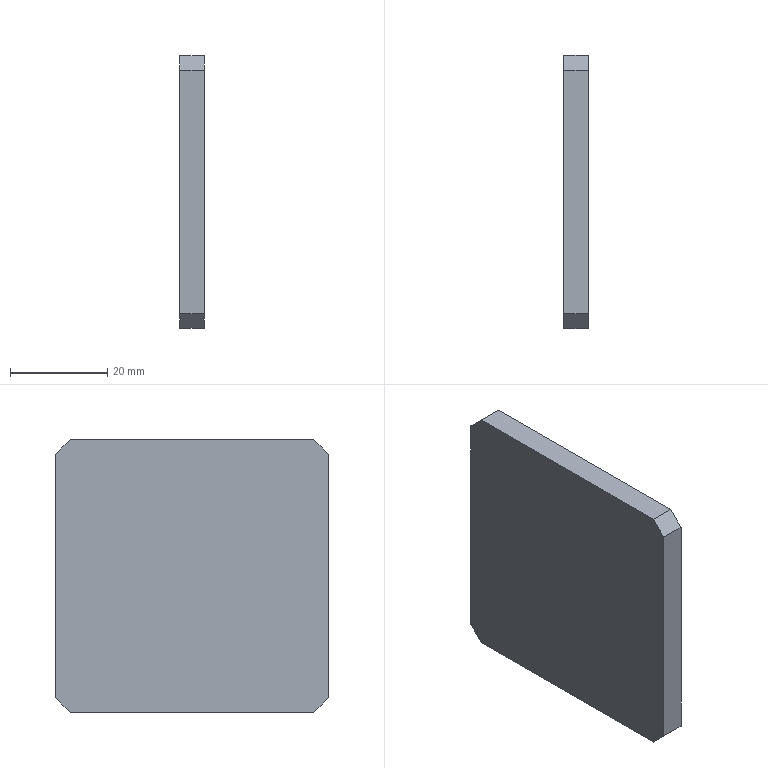Part | SolidWorks | features BaseBody 1 | 1 solid | 10 faces | box 5 x 56 x 56 mm | volume 15590 mm3 | plane 10
STEP:
#1=CARTESIAN_POINT('',(330.,1994.544,-22.));
#2=VERTEX_POINT('',#1);
#3=CARTESIAN_POINT('',(330.,1944.544,-22.));
#4=VERTEX_POINT('',#3);
#5=CARTESIAN_POINT('',(330.,2339.544,-22.));
#6=DIRECTION('',(0.,-1.,0.));
#7=VECTOR('',#6,1000.);
#8=LINE('',#5,#7);
#9=EDGE_CURVE('',#2,#4,#8,.T.);
#10=ORIENTED_EDGE('',*,*,#9,.T.);
#11=CARTESIAN_POINT('',(330.,1941.544,-25.));
#12=VERTEX_POINT('',#11);
#13=CARTESIAN_POINT('',(330.,1944.544,-22.));
#14=DIRECTION('',(0.,-0.7071,-0.7071));
#15=VECTOR('',#14,1000.);
#16=LINE('',#13,#15);
#17=EDGE_CURVE('',#4,#12,#16,.T.);
#18=ORIENTED_EDGE('',*,*,#17,.T.);
#19=CARTESIAN_POINT('',(330.,1941.544,-75.));
#20=VERTEX_POINT('',#19);
#21=CARTESIAN_POINT('',(330.,1941.544,-1550.));
#22=DIRECTION('',(0.,0.,-1.));
#23=VECTOR('',#22,1000.);
#24=LINE('',#21,#23);
#25=EDGE_CURVE('',#12,#20,#24,.T.);
#26=ORIENTED_EDGE('',*,*,#25,.T.);
#27=CARTESIAN_POINT('',(330.,1944.544,-78.));
#28=VERTEX_POINT('',#27);
#29=CARTESIAN_POINT('',(330.,1941.544,-75.));
#30=DIRECTION('',(0.,0.7071,-0.7071));
#31=VECTOR('',#30,1000.);
#32=LINE('',#29,#31);
#33=EDGE_CURVE('',#20,#28,#32,.T.);
#34=ORIENTED_EDGE('',*,*,#33,.T.);
#35=CARTESIAN_POINT('',(330.,1994.544,-78.));
#36=VERTEX_POINT('',#35);
#37=CARTESIAN_POINT('',(330.,2339.544,-78.));
#38=DIRECTION('',(0.,1.,0.));
#39=VECTOR('',#38,1000.);
#40=LINE('',#37,#39);
#41=EDGE_CURVE('',#28,#36,#40,.T.);
#42=ORIENTED_EDGE('',*,*,#41,.T.);
#43=CARTESIAN_POINT('',(330.,1997.544,-75.));
#44=VERTEX_POINT('',#43);
#45=CARTESIAN_POINT('',(330.,1994.544,-78.));
#46=DIRECTION('',(0.,0.7071,0.7071));
#47=VECTOR('',#46,1000.);
#48=LINE('',#45,#47);
#49=EDGE_CURVE('',#36,#44,#48,.T.);
#50=ORIENTED_EDGE('',*,*,#49,.T.);
#51=CARTESIAN_POINT('',(330.,1997.544,-25.));
#52=VERTEX_POINT('',#51);
#53=CARTESIAN_POINT('',(330.,1997.544,-1550.));
#54=DIRECTION('',(0.,0.,1.));
#55=VECTOR('',#54,1000.);
#56=LINE('',#53,#55);
#57=EDGE_CURVE('',#44,#52,#56,.T.);
#58=ORIENTED_EDGE('',*,*,#57,.T.);
#59=CARTESIAN_POINT('',(330.,1997.544,-25.));
#60=DIRECTION('',(0.,-0.7071,0.7071));
#61=VECTOR('',#60,1000.);
#62=LINE('',#59,#61);
#63=EDGE_CURVE('',#52,#2,#62,.T.);
#64=ORIENTED_EDGE('',*,*,#63,.T.);
#65=EDGE_LOOP('',(#10,#18,#26,#34,#42,#50,#58,#64));
#66=FACE_OUTER_BOUND('',#65,.T.);
#67=CARTESIAN_POINT('',(330.,2339.544,-1550.));
#68=DIRECTION('',(1.,0.,0.));
#69=DIRECTION('',(0.,0.,-1.));
#70=AXIS2_PLACEMENT_3D('',#67,#68,#69);
#71=PLANE('',#70);
#72=ADVANCED_FACE('',(#66),#71,.T.);
#73=ORIENTED_EDGE('',*,*,#17,.F.);
#74=CARTESIAN_POINT('',(325.,1944.544,-22.));
#75=VERTEX_POINT('',#74);
#76=CARTESIAN_POINT('',(330.,1944.544,-22.));
#77=DIRECTION('',(1.,0.,0.));
#78=VECTOR('',#77,1000.);
#79=LINE('',#76,#78);
#80=EDGE_CURVE('',#75,#4,#79,.T.);
#81=ORIENTED_EDGE('',*,*,#80,.F.);
#82=CARTESIAN_POINT('',(325.,1941.544,-25.));
#83=VERTEX_POINT('',#82);
#84=CARTESIAN_POINT('',(325.,1944.544,-22.));
#85=DIRECTION('',(0.,0.7071,0.7071));
#86=VECTOR('',#85,1000.);
#87=LINE('',#84,#86);
#88=EDGE_CURVE('',#83,#75,#87,.T.);
#89=ORIENTED_EDGE('',*,*,#88,.F.);
#90=CARTESIAN_POINT('',(330.,1941.544,-25.));
#91=DIRECTION('',(-1.,0.,0.));
#92=VECTOR('',#91,1000.);
#93=LINE('',#90,#92);
#94=EDGE_CURVE('',#12,#83,#93,.T.);
#95=ORIENTED_EDGE('',*,*,#94,.F.);
#96=EDGE_LOOP('',(#73,#81,#89,#95));
#97=FACE_OUTER_BOUND('',#96,.T.);
#98=CARTESIAN_POINT('',(330.,1944.544,-22.));
#99=DIRECTION('',(0.,0.7071,-0.7071));
#100=DIRECTION('',(0.,0.7071,0.7071));
#101=AXIS2_PLACEMENT_3D('',#98,#99,#100);
#102=PLANE('',#101);
#103=ADVANCED_FACE('',(#97),#102,.F.);
#104=ORIENTED_EDGE('',*,*,#9,.F.);
#105=CARTESIAN_POINT('',(325.,1994.544,-22.));
#106=VERTEX_POINT('',#105);
#107=CARTESIAN_POINT('',(330.,1994.544,-22.));
#108=DIRECTION('',(1.,0.,0.));
#109=VECTOR('',#108,1000.);
#110=LINE('',#107,#109);
#111=EDGE_CURVE('',#106,#2,#110,.T.);
#112=ORIENTED_EDGE('',*,*,#111,.F.);
#113=CARTESIAN_POINT('',(325.,1994.544,-22.));
#114=DIRECTION('',(0.,1.,0.));
#115=VECTOR('',#114,1000.);
#116=LINE('',#113,#115);
#117=EDGE_CURVE('',#75,#106,#116,.T.);
#118=ORIENTED_EDGE('',*,*,#117,.F.);
#119=ORIENTED_EDGE('',*,*,#80,.T.);
#120=EDGE_LOOP('',(#104,#112,#118,#119));
#121=FACE_OUTER_BOUND('',#120,.T.);
#122=CARTESIAN_POINT('',(330.,1994.544,-22.));
#123=DIRECTION('',(0.,0.,-1.));
#124=DIRECTION('',(-1.,0.,0.));
#125=AXIS2_PLACEMENT_3D('',#122,#123,#124);
#126=PLANE('',#125);
#127=ADVANCED_FACE('',(#121),#126,.F.);
#128=ORIENTED_EDGE('',*,*,#63,.F.);
#129=CARTESIAN_POINT('',(325.,1997.544,-25.));
#130=VERTEX_POINT('',#129);
#131=CARTESIAN_POINT('',(330.,1997.544,-25.));
#132=DIRECTION('',(1.,0.,0.));
#133=VECTOR('',#132,1000.);
#134=LINE('',#131,#133);
#135=EDGE_CURVE('',#130,#52,#134,.T.);
#136=ORIENTED_EDGE('',*,*,#135,.F.);
#137=CARTESIAN_POINT('',(325.,1997.544,-25.));
#138=DIRECTION('',(0.,0.7071,-0.7071));
#139=VECTOR('',#138,1000.);
#140=LINE('',#137,#139);
#141=EDGE_CURVE('',#106,#130,#140,.T.);
#142=ORIENTED_EDGE('',*,*,#141,.F.);
#143=ORIENTED_EDGE('',*,*,#111,.T.);
#144=EDGE_LOOP('',(#128,#136,#142,#143));
#145=FACE_OUTER_BOUND('',#144,.T.);
#146=CARTESIAN_POINT('',(330.,1997.544,-25.));
#147=DIRECTION('',(0.,-0.7071,-0.7071));
#148=DIRECTION('',(0.,0.7071,-0.7071));
#149=AXIS2_PLACEMENT_3D('',#146,#147,#148);
#150=PLANE('',#149);
#151=ADVANCED_FACE('',(#145),#150,.F.);
#152=ORIENTED_EDGE('',*,*,#57,.F.);
#153=CARTESIAN_POINT('',(325.,1997.544,-75.));
#154=VERTEX_POINT('',#153);
#155=CARTESIAN_POINT('',(330.,1997.544,-75.));
#156=DIRECTION('',(1.,0.,0.));
#157=VECTOR('',#156,1000.);
#158=LINE('',#155,#157);
#159=EDGE_CURVE('',#154,#44,#158,.T.);
#160=ORIENTED_EDGE('',*,*,#159,.F.);
#161=CARTESIAN_POINT('',(325.,1997.544,-75.));
#162=DIRECTION('',(0.,0.,-1.));
#163=VECTOR('',#162,1000.);
#164=LINE('',#161,#163);
#165=EDGE_CURVE('',#130,#154,#164,.T.);
#166=ORIENTED_EDGE('',*,*,#165,.F.);
#167=ORIENTED_EDGE('',*,*,#135,.T.);
#168=EDGE_LOOP('',(#152,#160,#166,#167));
#169=FACE_OUTER_BOUND('',#168,.T.);
#170=CARTESIAN_POINT('',(330.,1997.544,-75.));
#171=DIRECTION('',(0.,-1.,0.));
#172=DIRECTION('',(0.,0.,-1.));
#173=AXIS2_PLACEMENT_3D('',#170,#171,#172);
#174=PLANE('',#173);
#175=ADVANCED_FACE('',(#169),#174,.F.);
#176=ORIENTED_EDGE('',*,*,#49,.F.);
#177=CARTESIAN_POINT('',(325.,1994.544,-78.));
#178=VERTEX_POINT('',#177);
#179=CARTESIAN_POINT('',(330.,1994.544,-78.));
#180=DIRECTION('',(1.,0.,0.));
#181=VECTOR('',#180,1000.);
#182=LINE('',#179,#181);
#183=EDGE_CURVE('',#178,#36,#182,.T.);
#184=ORIENTED_EDGE('',*,*,#183,.F.);
#185=CARTESIAN_POINT('',(325.,1994.544,-78.));
#186=DIRECTION('',(0.,-0.7071,-0.7071));
#187=VECTOR('',#186,1000.);
#188=LINE('',#185,#187);
#189=EDGE_CURVE('',#154,#178,#188,.T.);
#190=ORIENTED_EDGE('',*,*,#189,.F.);
#191=ORIENTED_EDGE('',*,*,#159,.T.);
#192=EDGE_LOOP('',(#176,#184,#190,#191));
#193=FACE_OUTER_BOUND('',#192,.T.);
#194=CARTESIAN_POINT('',(330.,1994.544,-78.));
#195=DIRECTION('',(0.,-0.7071,0.7071));
#196=DIRECTION('',(0.,-0.7071,-0.7071));
#197=AXIS2_PLACEMENT_3D('',#194,#195,#196);
#198=PLANE('',#197);
#199=ADVANCED_FACE('',(#193),#198,.F.);
#200=ORIENTED_EDGE('',*,*,#41,.F.);
#201=CARTESIAN_POINT('',(325.,1944.544,-78.));
#202=VERTEX_POINT('',#201);
#203=CARTESIAN_POINT('',(330.,1944.544,-78.));
#204=DIRECTION('',(1.,0.,0.));
#205=VECTOR('',#204,1000.);
#206=LINE('',#203,#205);
#207=EDGE_CURVE('',#202,#28,#206,.T.);
#208=ORIENTED_EDGE('',*,*,#207,.F.);
#209=CARTESIAN_POINT('',(325.,1944.544,-78.));
#210=DIRECTION('',(0.,-1.,0.));
#211=VECTOR('',#210,1000.);
#212=LINE('',#209,#211);
#213=EDGE_CURVE('',#178,#202,#212,.T.);
#214=ORIENTED_EDGE('',*,*,#213,.F.);
#215=ORIENTED_EDGE('',*,*,#183,.T.);
#216=EDGE_LOOP('',(#200,#208,#214,#215));
#217=FACE_OUTER_BOUND('',#216,.T.);
#218=CARTESIAN_POINT('',(330.,1944.544,-78.));
#219=DIRECTION('',(0.,0.,1.));
#220=DIRECTION('',(1.,0.,0.));
#221=AXIS2_PLACEMENT_3D('',#218,#219,#220);
#222=PLANE('',#221);
#223=ADVANCED_FACE('',(#217),#222,.F.);
#224=ORIENTED_EDGE('',*,*,#33,.F.);
#225=CARTESIAN_POINT('',(325.,1941.544,-75.));
#226=VERTEX_POINT('',#225);
#227=CARTESIAN_POINT('',(330.,1941.544,-75.));
#228=DIRECTION('',(1.,0.,0.));
#229=VECTOR('',#228,1000.);
#230=LINE('',#227,#229);
#231=EDGE_CURVE('',#226,#20,#230,.T.);
#232=ORIENTED_EDGE('',*,*,#231,.F.);
#233=CARTESIAN_POINT('',(325.,1941.544,-75.));
#234=DIRECTION('',(0.,-0.7071,0.7071));
#235=VECTOR('',#234,1000.);
#236=LINE('',#233,#235);
#237=EDGE_CURVE('',#202,#226,#236,.T.);
#238=ORIENTED_EDGE('',*,*,#237,.F.);
#239=ORIENTED_EDGE('',*,*,#207,.T.);
#240=EDGE_LOOP('',(#224,#232,#238,#239));
#241=FACE_OUTER_BOUND('',#240,.T.);
#242=CARTESIAN_POINT('',(330.,1941.544,-75.));
#243=DIRECTION('',(0.,0.7071,0.7071));
#244=DIRECTION('',(0.,-0.7071,0.7071));
#245=AXIS2_PLACEMENT_3D('',#242,#243,#244);
#246=PLANE('',#245);
#247=ADVANCED_FACE('',(#241),#246,.F.);
#248=ORIENTED_EDGE('',*,*,#25,.F.);
#249=ORIENTED_EDGE('',*,*,#94,.T.);
#250=CARTESIAN_POINT('',(325.,1941.544,-25.));
#251=DIRECTION('',(0.,0.,1.));
#252=VECTOR('',#251,1000.);
#253=LINE('',#250,#252);
#254=EDGE_CURVE('',#226,#83,#253,.T.);
#255=ORIENTED_EDGE('',*,*,#254,.F.);
#256=ORIENTED_EDGE('',*,*,#231,.T.);
#257=EDGE_LOOP('',(#248,#249,#255,#256));
#258=FACE_OUTER_BOUND('',#257,.T.);
#259=CARTESIAN_POINT('',(330.,1941.544,-25.));
#260=DIRECTION('',(0.,1.,0.));
#261=DIRECTION('',(0.,0.,1.));
#262=AXIS2_PLACEMENT_3D('',#259,#260,#261);
#263=PLANE('',#262);
#264=ADVANCED_FACE('',(#258),#263,.F.);
#265=ORIENTED_EDGE('',*,*,#141,.T.);
#266=ORIENTED_EDGE('',*,*,#165,.T.);
#267=ORIENTED_EDGE('',*,*,#189,.T.);
#268=ORIENTED_EDGE('',*,*,#213,.T.);
#269=ORIENTED_EDGE('',*,*,#237,.T.);
#270=ORIENTED_EDGE('',*,*,#254,.T.);
#271=ORIENTED_EDGE('',*,*,#88,.T.);
#272=ORIENTED_EDGE('',*,*,#117,.T.);
#273=EDGE_LOOP('',(#265,#266,#267,#268,#269,#270,#271,#272));
#274=FACE_OUTER_BOUND('',#273,.T.);
#275=CARTESIAN_POINT('',(325.,2339.544,-1550.));
#276=DIRECTION('',(1.,0.,0.));
#277=DIRECTION('',(0.,0.,-1.));
#278=AXIS2_PLACEMENT_3D('',#275,#276,#277);
#279=PLANE('',#278);
#280=ADVANCED_FACE('',(#274),#279,.F.);
#281=CLOSED_SHELL('',(#72,#103,#127,#151,#175,#199,#223,#247,#264,#280));
#282=MANIFOLD_SOLID_BREP('',#281);
#283=CARTESIAN_POINT('',(0.,0.,0.));
#284=DIRECTION('',(0.,0.,1.));
#285=DIRECTION('',(1.,0.,0.));
#286=AXIS2_PLACEMENT_3D('',#283,#284,#285);
#287=(LENGTH_UNIT()NAMED_UNIT(*)SI_UNIT(.MILLI.,.METRE.));
#288=UNCERTAINTY_MEASURE_WITH_UNIT(LENGTH_MEASURE(0.00001),#287,'','');
#289=(NAMED_UNIT(*)PLANE_ANGLE_UNIT()SI_UNIT($,.RADIAN.));
#290=(NAMED_UNIT(*)SI_UNIT($,.STERADIAN.)SOLID_ANGLE_UNIT());
#291=(GEOMETRIC_REPRESENTATION_CONTEXT(3)GLOBAL_UNCERTAINTY_ASSIGNED_CONTEXT((#288))GLOBAL_UNIT_ASSIGNED_CONTEXT((#287,#289,#290))REPRESENTATION_CONTEXT('',''));
#292=ADVANCED_BREP_SHAPE_REPRESENTATION('',(#282,#286),#291);